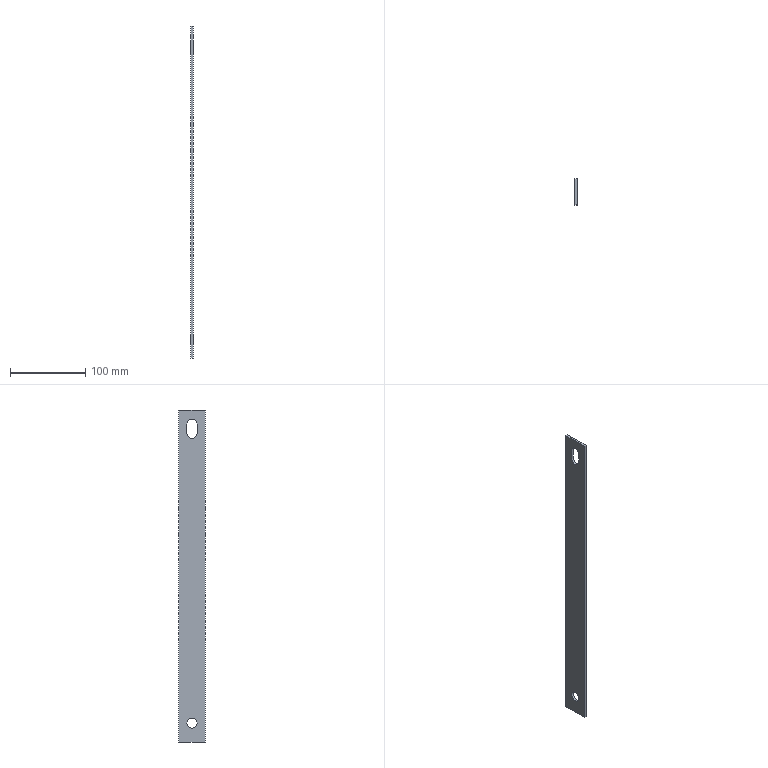Part | NX | features solid 2 | 1 solid | 11 faces | box 3 x 35 x 440 mm | volume 44835 mm3 | plane 8 | cylinder 3 | commonest cylinder face diameters 13.5 x3
STEP:
#1=CARTESIAN_POINT('',(-1160.,-486.75,286.25));
#2=VERTEX_POINT('',#1);
#3=CARTESIAN_POINT('',(-1160.,-473.25,286.25));
#4=VERTEX_POINT('',#3);
#5=CARTESIAN_POINT('',(-1160.,-480.,286.25));
#6=DIRECTION('',(-1.,0.,0.));
#7=DIRECTION('',(0.,-1.,0.));
#8=AXIS2_PLACEMENT_3D('',#5,#6,#7);
#9=CIRCLE('',#8,6.75);
#10=EDGE_CURVE('',#2,#4,#9,.T.);
#11=ORIENTED_EDGE('',*,*,#10,.F.);
#12=CARTESIAN_POINT('',(-1163.,-486.75,286.25));
#13=VERTEX_POINT('',#12);
#14=CARTESIAN_POINT('',(-1163.,-486.75,286.25));
#15=DIRECTION('',(1.,0.,0.));
#16=VECTOR('',#15,1000.);
#17=LINE('',#14,#16);
#18=EDGE_CURVE('',#13,#2,#17,.T.);
#19=ORIENTED_EDGE('',*,*,#18,.F.);
#20=CARTESIAN_POINT('',(-1163.,-473.25,286.25));
#21=VERTEX_POINT('',#20);
#22=CARTESIAN_POINT('',(-1163.,-480.,286.25));
#23=DIRECTION('',(-1.,0.,0.));
#24=DIRECTION('',(0.,-1.,0.));
#25=AXIS2_PLACEMENT_3D('',#22,#23,#24);
#26=CIRCLE('',#25,6.75);
#27=EDGE_CURVE('',#13,#21,#26,.T.);
#28=ORIENTED_EDGE('',*,*,#27,.T.);
#29=CARTESIAN_POINT('',(-1163.,-473.25,286.25));
#30=DIRECTION('',(1.,0.,0.));
#31=VECTOR('',#30,1000.);
#32=LINE('',#29,#31);
#33=EDGE_CURVE('',#21,#4,#32,.T.);
#34=ORIENTED_EDGE('',*,*,#33,.T.);
#35=EDGE_LOOP('',(#11,#19,#28,#34));
#36=FACE_BOUND('',#35,.T.);
#37=CARTESIAN_POINT('',(-1163.,-480.,286.25));
#38=DIRECTION('',(1.,0.,0.));
#39=DIRECTION('',(0.,-1.,0.));
#40=AXIS2_PLACEMENT_3D('',#37,#38,#39);
#41=CYLINDRICAL_SURFACE('',#40,6.75);
#42=ADVANCED_FACE('',(#36),#41,.F.);
#43=CARTESIAN_POINT('',(-1160.,-486.75,273.75));
#44=VERTEX_POINT('',#43);
#45=CARTESIAN_POINT('',(-1160.,-486.75,286.25));
#46=DIRECTION('',(0.,0.,-1.));
#47=VECTOR('',#46,1000.);
#48=LINE('',#45,#47);
#49=EDGE_CURVE('',#2,#44,#48,.T.);
#50=ORIENTED_EDGE('',*,*,#49,.T.);
#51=CARTESIAN_POINT('',(-1163.,-486.75,273.75));
#52=VERTEX_POINT('',#51);
#53=CARTESIAN_POINT('',(-1163.,-486.75,273.75));
#54=DIRECTION('',(1.,0.,0.));
#55=VECTOR('',#54,1000.);
#56=LINE('',#53,#55);
#57=EDGE_CURVE('',#52,#44,#56,.T.);
#58=ORIENTED_EDGE('',*,*,#57,.F.);
#59=CARTESIAN_POINT('',(-1163.,-486.75,286.25));
#60=DIRECTION('',(0.,0.,-1.));
#61=VECTOR('',#60,1000.);
#62=LINE('',#59,#61);
#63=EDGE_CURVE('',#13,#52,#62,.T.);
#64=ORIENTED_EDGE('',*,*,#63,.F.);
#65=ORIENTED_EDGE('',*,*,#18,.T.);
#66=EDGE_LOOP('',(#50,#58,#64,#65));
#67=FACE_BOUND('',#66,.T.);
#68=CARTESIAN_POINT('',(-1163.,-486.75,286.25));
#69=DIRECTION('',(0.,1.,0.));
#70=DIRECTION('',(1.,0.,0.));
#71=AXIS2_PLACEMENT_3D('',#68,#69,#70);
#72=PLANE('',#71);
#73=ADVANCED_FACE('',(#67),#72,.T.);
#74=CARTESIAN_POINT('',(-1160.,-473.25,273.75));
#75=VERTEX_POINT('',#74);
#76=CARTESIAN_POINT('',(-1160.,-480.,273.75));
#77=DIRECTION('',(-1.,0.,0.));
#78=DIRECTION('',(0.,-1.,0.));
#79=AXIS2_PLACEMENT_3D('',#76,#77,#78);
#80=CIRCLE('',#79,6.75);
#81=EDGE_CURVE('',#75,#44,#80,.T.);
#82=ORIENTED_EDGE('',*,*,#81,.F.);
#83=CARTESIAN_POINT('',(-1163.,-473.25,273.75));
#84=VERTEX_POINT('',#83);
#85=CARTESIAN_POINT('',(-1163.,-473.25,273.75));
#86=DIRECTION('',(1.,0.,0.));
#87=VECTOR('',#86,1000.);
#88=LINE('',#85,#87);
#89=EDGE_CURVE('',#84,#75,#88,.T.);
#90=ORIENTED_EDGE('',*,*,#89,.F.);
#91=CARTESIAN_POINT('',(-1163.,-480.,273.75));
#92=DIRECTION('',(-1.,0.,0.));
#93=DIRECTION('',(0.,-1.,0.));
#94=AXIS2_PLACEMENT_3D('',#91,#92,#93);
#95=CIRCLE('',#94,6.75);
#96=EDGE_CURVE('',#84,#52,#95,.T.);
#97=ORIENTED_EDGE('',*,*,#96,.T.);
#98=ORIENTED_EDGE('',*,*,#57,.T.);
#99=EDGE_LOOP('',(#82,#90,#97,#98));
#100=FACE_BOUND('',#99,.T.);
#101=CARTESIAN_POINT('',(-1163.,-480.,273.75));
#102=DIRECTION('',(1.,0.,0.));
#103=DIRECTION('',(0.,-1.,0.));
#104=AXIS2_PLACEMENT_3D('',#101,#102,#103);
#105=CYLINDRICAL_SURFACE('',#104,6.75);
#106=ADVANCED_FACE('',(#100),#105,.F.);
#107=CARTESIAN_POINT('',(-1160.,-497.5,-135.));
#108=VERTEX_POINT('',#107);
#109=CARTESIAN_POINT('',(-1160.,-497.5,305.));
#110=VERTEX_POINT('',#109);
#111=CARTESIAN_POINT('',(-1160.,-497.5,5.));
#112=DIRECTION('',(0.,0.,1.));
#113=VECTOR('',#112,1000.);
#114=LINE('',#111,#113);
#115=EDGE_CURVE('',#108,#110,#114,.T.);
#116=ORIENTED_EDGE('',*,*,#115,.T.);
#117=CARTESIAN_POINT('',(-1163.,-497.5,305.));
#118=VERTEX_POINT('',#117);
#119=CARTESIAN_POINT('',(-1163.,-497.5,305.));
#120=DIRECTION('',(1.,0.,0.));
#121=VECTOR('',#120,1000.);
#122=LINE('',#119,#121);
#123=EDGE_CURVE('',#118,#110,#122,.T.);
#124=ORIENTED_EDGE('',*,*,#123,.F.);
#125=CARTESIAN_POINT('',(-1163.,-497.5,-135.));
#126=VERTEX_POINT('',#125);
#127=CARTESIAN_POINT('',(-1163.,-497.5,5.));
#128=DIRECTION('',(0.,0.,1.));
#129=VECTOR('',#128,1000.);
#130=LINE('',#127,#129);
#131=EDGE_CURVE('',#126,#118,#130,.T.);
#132=ORIENTED_EDGE('',*,*,#131,.F.);
#133=CARTESIAN_POINT('',(-1163.,-497.5,-135.));
#134=DIRECTION('',(1.,0.,0.));
#135=VECTOR('',#134,1000.);
#136=LINE('',#133,#135);
#137=EDGE_CURVE('',#126,#108,#136,.T.);
#138=ORIENTED_EDGE('',*,*,#137,.T.);
#139=EDGE_LOOP('',(#116,#124,#132,#138));
#140=FACE_BOUND('',#139,.T.);
#141=CARTESIAN_POINT('',(-1163.,-497.5,5.));
#142=DIRECTION('',(0.,-1.,0.));
#143=DIRECTION('',(0.,0.,1.));
#144=AXIS2_PLACEMENT_3D('',#141,#142,#143);
#145=PLANE('',#144);
#146=ADVANCED_FACE('',(#140),#145,.T.);
#147=CARTESIAN_POINT('',(-1160.,-462.5,305.));
#148=VERTEX_POINT('',#147);
#149=CARTESIAN_POINT('',(-1160.,-497.5,305.));
#150=DIRECTION('',(0.,1.,0.));
#151=VECTOR('',#150,1000.);
#152=LINE('',#149,#151);
#153=EDGE_CURVE('',#110,#148,#152,.T.);
#154=ORIENTED_EDGE('',*,*,#153,.T.);
#155=CARTESIAN_POINT('',(-1163.,-462.5,305.));
#156=VERTEX_POINT('',#155);
#157=CARTESIAN_POINT('',(-1163.,-462.5,305.));
#158=DIRECTION('',(1.,0.,0.));
#159=VECTOR('',#158,1000.);
#160=LINE('',#157,#159);
#161=EDGE_CURVE('',#156,#148,#160,.T.);
#162=ORIENTED_EDGE('',*,*,#161,.F.);
#163=CARTESIAN_POINT('',(-1163.,-497.5,305.));
#164=DIRECTION('',(0.,1.,0.));
#165=VECTOR('',#164,1000.);
#166=LINE('',#163,#165);
#167=EDGE_CURVE('',#118,#156,#166,.T.);
#168=ORIENTED_EDGE('',*,*,#167,.F.);
#169=ORIENTED_EDGE('',*,*,#123,.T.);
#170=EDGE_LOOP('',(#154,#162,#168,#169));
#171=FACE_BOUND('',#170,.T.);
#172=CARTESIAN_POINT('',(-1163.,-497.5,305.));
#173=DIRECTION('',(0.,0.,1.));
#174=DIRECTION('',(1.,0.,0.));
#175=AXIS2_PLACEMENT_3D('',#172,#173,#174);
#176=PLANE('',#175);
#177=ADVANCED_FACE('',(#171),#176,.T.);
#178=CARTESIAN_POINT('',(-1160.,-462.5,-135.));
#179=VERTEX_POINT('',#178);
#180=CARTESIAN_POINT('',(-1160.,-462.5,305.));
#181=DIRECTION('',(0.,0.,-1.));
#182=VECTOR('',#181,1000.);
#183=LINE('',#180,#182);
#184=EDGE_CURVE('',#148,#179,#183,.T.);
#185=ORIENTED_EDGE('',*,*,#184,.T.);
#186=CARTESIAN_POINT('',(-1163.,-462.5,-135.));
#187=VERTEX_POINT('',#186);
#188=CARTESIAN_POINT('',(-1163.,-462.5,-135.));
#189=DIRECTION('',(1.,0.,0.));
#190=VECTOR('',#189,1000.);
#191=LINE('',#188,#190);
#192=EDGE_CURVE('',#187,#179,#191,.T.);
#193=ORIENTED_EDGE('',*,*,#192,.F.);
#194=CARTESIAN_POINT('',(-1163.,-462.5,305.));
#195=DIRECTION('',(0.,0.,-1.));
#196=VECTOR('',#195,1000.);
#197=LINE('',#194,#196);
#198=EDGE_CURVE('',#156,#187,#197,.T.);
#199=ORIENTED_EDGE('',*,*,#198,.F.);
#200=ORIENTED_EDGE('',*,*,#161,.T.);
#201=EDGE_LOOP('',(#185,#193,#199,#200));
#202=FACE_BOUND('',#201,.T.);
#203=CARTESIAN_POINT('',(-1163.,-462.5,305.));
#204=DIRECTION('',(0.,1.,0.));
#205=DIRECTION('',(0.,0.,-1.));
#206=AXIS2_PLACEMENT_3D('',#203,#204,#205);
#207=PLANE('',#206);
#208=ADVANCED_FACE('',(#202),#207,.T.);
#209=CARTESIAN_POINT('',(-1163.,-486.75,-110.));
#210=VERTEX_POINT('',#209);
#211=CARTESIAN_POINT('',(-1163.,-480.,-110.));
#212=DIRECTION('',(-1.,0.,0.));
#213=DIRECTION('',(0.,-1.,0.));
#214=AXIS2_PLACEMENT_3D('',#211,#212,#213);
#215=CIRCLE('',#214,6.75);
#216=EDGE_CURVE('',#210,#210,#215,.T.);
#217=ORIENTED_EDGE('',*,*,#216,.T.);
#218=EDGE_LOOP('',(#217));
#219=FACE_BOUND('',#218,.T.);
#220=CARTESIAN_POINT('',(-1160.,-486.75,-110.));
#221=VERTEX_POINT('',#220);
#222=CARTESIAN_POINT('',(-1160.,-480.,-110.));
#223=DIRECTION('',(-1.,0.,0.));
#224=DIRECTION('',(0.,-1.,0.));
#225=AXIS2_PLACEMENT_3D('',#222,#223,#224);
#226=CIRCLE('',#225,6.75);
#227=EDGE_CURVE('',#221,#221,#226,.T.);
#228=ORIENTED_EDGE('',*,*,#227,.F.);
#229=EDGE_LOOP('',(#228));
#230=FACE_BOUND('',#229,.T.);
#231=CARTESIAN_POINT('',(-1163.,-480.,-110.));
#232=DIRECTION('',(1.,0.,0.));
#233=DIRECTION('',(0.,-1.,0.));
#234=AXIS2_PLACEMENT_3D('',#231,#232,#233);
#235=CYLINDRICAL_SURFACE('',#234,6.75);
#236=ADVANCED_FACE('',(#219,#230),#235,.F.);
#237=CARTESIAN_POINT('',(-1160.,-462.5,-135.));
#238=DIRECTION('',(0.,-1.,0.));
#239=VECTOR('',#238,1000.);
#240=LINE('',#237,#239);
#241=EDGE_CURVE('',#179,#108,#240,.T.);
#242=ORIENTED_EDGE('',*,*,#241,.T.);
#243=ORIENTED_EDGE('',*,*,#137,.F.);
#244=CARTESIAN_POINT('',(-1163.,-462.5,-135.));
#245=DIRECTION('',(0.,-1.,0.));
#246=VECTOR('',#245,1000.);
#247=LINE('',#244,#246);
#248=EDGE_CURVE('',#187,#126,#247,.T.);
#249=ORIENTED_EDGE('',*,*,#248,.F.);
#250=ORIENTED_EDGE('',*,*,#192,.T.);
#251=EDGE_LOOP('',(#242,#243,#249,#250));
#252=FACE_BOUND('',#251,.T.);
#253=CARTESIAN_POINT('',(-1163.,-462.5,-135.));
#254=DIRECTION('',(0.,0.,-1.));
#255=DIRECTION('',(-1.,0.,0.));
#256=AXIS2_PLACEMENT_3D('',#253,#254,#255);
#257=PLANE('',#256);
#258=ADVANCED_FACE('',(#252),#257,.T.);
#259=CARTESIAN_POINT('',(-1160.,-473.25,273.75));
#260=DIRECTION('',(0.,0.,1.));
#261=VECTOR('',#260,1000.);
#262=LINE('',#259,#261);
#263=EDGE_CURVE('',#75,#4,#262,.T.);
#264=ORIENTED_EDGE('',*,*,#263,.T.);
#265=ORIENTED_EDGE('',*,*,#33,.F.);
#266=CARTESIAN_POINT('',(-1163.,-473.25,273.75));
#267=DIRECTION('',(0.,0.,1.));
#268=VECTOR('',#267,1000.);
#269=LINE('',#266,#268);
#270=EDGE_CURVE('',#84,#21,#269,.T.);
#271=ORIENTED_EDGE('',*,*,#270,.F.);
#272=ORIENTED_EDGE('',*,*,#89,.T.);
#273=EDGE_LOOP('',(#264,#265,#271,#272));
#274=FACE_BOUND('',#273,.T.);
#275=CARTESIAN_POINT('',(-1163.,-473.25,273.75));
#276=DIRECTION('',(0.,-1.,0.));
#277=DIRECTION('',(-1.,0.,0.));
#278=AXIS2_PLACEMENT_3D('',#275,#276,#277);
#279=PLANE('',#278);
#280=ADVANCED_FACE('',(#274),#279,.T.);
#281=ORIENTED_EDGE('',*,*,#131,.T.);
#282=ORIENTED_EDGE('',*,*,#167,.T.);
#283=ORIENTED_EDGE('',*,*,#198,.T.);
#284=ORIENTED_EDGE('',*,*,#248,.T.);
#285=EDGE_LOOP('',(#281,#282,#283,#284));
#286=FACE_BOUND('',#285,.T.);
#287=ORIENTED_EDGE('',*,*,#216,.F.);
#288=EDGE_LOOP('',(#287));
#289=FACE_BOUND('',#288,.T.);
#290=ORIENTED_EDGE('',*,*,#27,.F.);
#291=ORIENTED_EDGE('',*,*,#63,.T.);
#292=ORIENTED_EDGE('',*,*,#96,.F.);
#293=ORIENTED_EDGE('',*,*,#270,.T.);
#294=EDGE_LOOP('',(#290,#291,#292,#293));
#295=FACE_BOUND('',#294,.T.);
#296=CARTESIAN_POINT('',(-1163.,-497.5,305.));
#297=DIRECTION('',(1.,0.,0.));
#298=DIRECTION('',(0.,-1.,0.));
#299=AXIS2_PLACEMENT_3D('',#296,#297,#298);
#300=PLANE('',#299);
#301=ADVANCED_FACE('',(#286,#289,#295),#300,.F.);
#302=ORIENTED_EDGE('',*,*,#115,.F.);
#303=ORIENTED_EDGE('',*,*,#241,.F.);
#304=ORIENTED_EDGE('',*,*,#184,.F.);
#305=ORIENTED_EDGE('',*,*,#153,.F.);
#306=EDGE_LOOP('',(#302,#303,#304,#305));
#307=FACE_BOUND('',#306,.T.);
#308=ORIENTED_EDGE('',*,*,#227,.T.);
#309=EDGE_LOOP('',(#308));
#310=FACE_BOUND('',#309,.T.);
#311=ORIENTED_EDGE('',*,*,#10,.T.);
#312=ORIENTED_EDGE('',*,*,#263,.F.);
#313=ORIENTED_EDGE('',*,*,#81,.T.);
#314=ORIENTED_EDGE('',*,*,#49,.F.);
#315=EDGE_LOOP('',(#311,#312,#313,#314));
#316=FACE_BOUND('',#315,.T.);
#317=CARTESIAN_POINT('',(-1160.,-497.5,305.));
#318=DIRECTION('',(1.,0.,0.));
#319=DIRECTION('',(0.,-1.,0.));
#320=AXIS2_PLACEMENT_3D('',#317,#318,#319);
#321=PLANE('',#320);
#322=ADVANCED_FACE('',(#307,#310,#316),#321,.T.);
#323=CLOSED_SHELL('',(#42,#73,#106,#146,#177,#208,#236,#258,#280,#301,#322));
#324=MANIFOLD_SOLID_BREP('',#323);
#325=(LENGTH_UNIT()NAMED_UNIT(*)SI_UNIT(.MILLI.,.METRE.));
#326=UNCERTAINTY_MEASURE_WITH_UNIT(LENGTH_MEASURE(0.00001),#325,'','');
#327=(NAMED_UNIT(*)PLANE_ANGLE_UNIT()SI_UNIT($,.RADIAN.));
#328=(NAMED_UNIT(*)SI_UNIT($,.STERADIAN.)SOLID_ANGLE_UNIT());
#329=(GEOMETRIC_REPRESENTATION_CONTEXT(3)GLOBAL_UNCERTAINTY_ASSIGNED_CONTEXT((#326))GLOBAL_UNIT_ASSIGNED_CONTEXT((#325,#327,#328))REPRESENTATION_CONTEXT('',''));
#330=ADVANCED_BREP_SHAPE_REPRESENTATION('',(#324),#329);